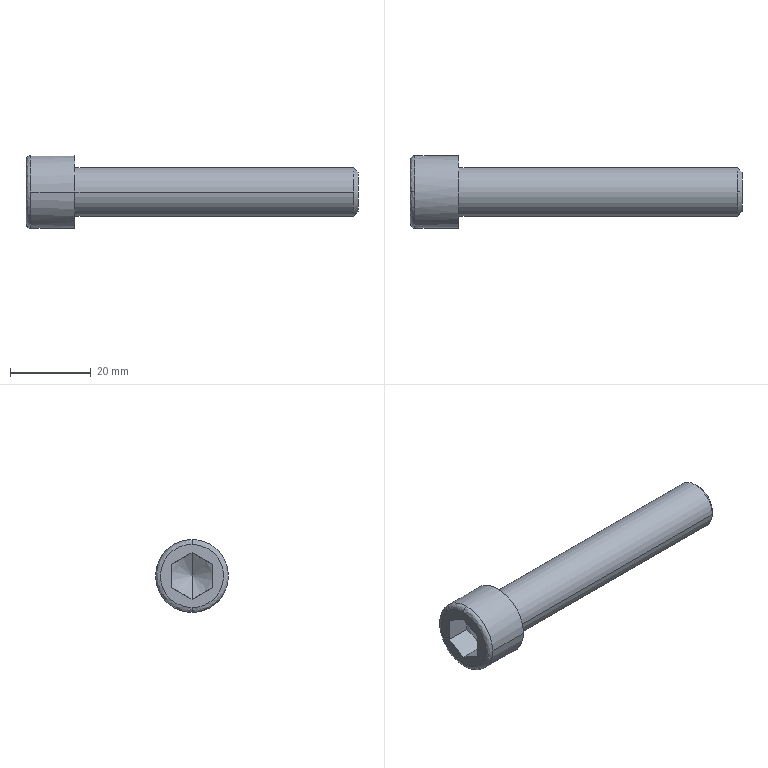Part | STEP file | DIN 912 - replaced by DIN EN ISO 4762 M12 x 70 | 1 solid | 21 faces | box 82 x 18 x 18 mm | volume 10300 mm3 | plane 9 | spline 4 | cylinder 4 | cone 4 | commonest cylinder face diameters 12 x2 18 x2